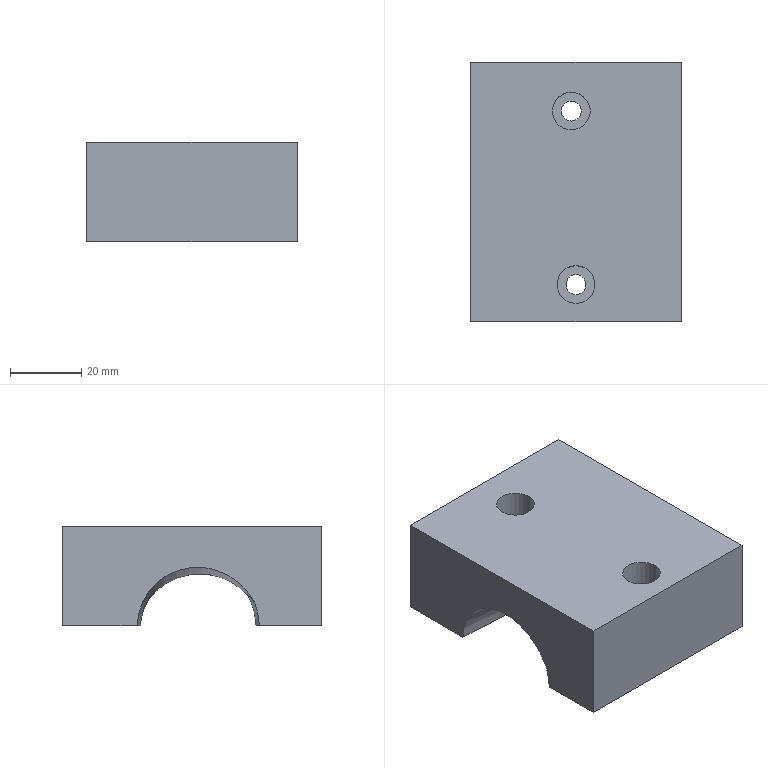NC program | NX | posted with a generic post | part box 59.014 x 72.744 x 27.972 mm
Whole program:
N10 G17 G21 G94 G90
(FLOOR_WALL , TOOL : D63)
N12 T03 M6
N14 G54
N16 G17 G0 G90 X73.872 Y0. S6500 M3
N18 G43 Z30. H3
N20 Z3.
N22 G94 G1 Z0. F1500.
N24 X70.872
N26 X-70.872
N28 X-73.872
N30 Z3.
N32 G0 Z30.
N34 M5
(DRILLING , TOOL : D6A45)
N36 T01 M6
N38 G54
N40 G17 G0 G90 X25.98 Y0. S5000 M3
N42 G43 Z30. H1
N44 G94 G81 G98 Z-1. F250. R3.
N46 X-22.701 Y-1.319
N48 G80
N50 G0 X-22.701 Y-1.319 Z30.
N52 M5
(DRILLING_COPY_COPY , TOOL : 5.6ZT)
N54 T20 M6
N56 G54
N58 G17 G0 G90 X-22.701 Y-1.319 S2000 M3
N60 G43 Z30. H20
N62 G94 G83 G98 Z-31.154 F150. Q3. R3.
N64 X25.98 Y0.
N66 G80
N68 G0 X25.98 Y0. Z30.
N70 M5
(HOLE_MILLING , TOOL : D6)
N72 T16 M6
N74 G54
N76 G17 G0 G90 X-22.701 Y-1.319 S9500 M3
N78 G43 Z30. H16
N80 Z0.5
N82 G94 G3 X-21.551 Y-0.169 R1.15 F1450.
N84 X-22.701 Y0.981 R1.15
N86 X-22.701 Y0.981 Z0. I0. J-2.3
N88 X-22.701 Y0.981 Z-0.5 I0. J-2.3
N90 X-22.701 Y0.981 Z-1. I0. J-2.3
N92 X-22.701 Y0.981 Z-1.5 I0. J-2.3
N94 X-22.701 Y0.981 Z-2. I0. J-2.3
N96 X-22.701 Y0.981 Z-2.5 I0. J-2.3
N98 X-22.701 Y0.981 Z-3. I0. J-2.3
N100 X-22.701 Y0.981 Z-3.5 I0. J-2.3
N102 X-22.701 Y0.981 Z-4. I0. J-2.3
N104 X-22.701 Y0.981 Z-4.5 I0. J-2.3
N106 X-22.701 Y0.981 Z-5. I0. J-2.3
N108 X-22.701 Y0.981 Z-5.5 I0. J-2.3
N110 X-22.701 Y0.981 Z-6. I0. J-2.3
N112 X-22.701 Y0.981 Z-6.5 I0. J-2.3
N114 X-22.701 Y0.981 Z-7. I0. J-2.3
N116 X-22.701 Y0.981 Z-7.5 I0. J-2.3
N118 X-22.701 Y0.981 Z-8. I0. J-2.3
N120 X-22.701 Y0.981 Z-8.5 I0. J-2.3
N122 X-22.701 Y0.981 Z-9. I0. J-2.3
N124 X-22.701 Y0.981 Z-9.5 I0. J-2.3
N126 X-22.701 Y0.981 Z-10. I0. J-2.3
N128 X-22.701 Y0.981 Z-10.5 I0. J-2.3
N130 X-22.701 Y0.981 Z-11. I0. J-2.3
N132 X-22.701 Y0.981 Z-11.5 I0. J-2.3
N134 X-22.701 Y0.981 Z-12. I0. J-2.3
N136 X-22.701 Y0.981 Z-12.5 I0. J-2.3
N138 X-22.701 Y0.981 Z-13. I0. J-2.3
N140 X-22.701 Y0.981 Z-13.5 I0. J-2.3
N142 X-22.701 Y0.981 Z-14. I0. J-2.3
N144 X-22.701 Y0.981 Z-14.5 I0. J-2.3
N146 X-22.701 Y0.981 Z-15. I0. J-2.3
N148 X-22.701 Y0.981 Z-15.5 I0. J-2.3
N150 X-22.701 Y0.981 Z-16. I0. J-2.3
N152 X-22.701 Y0.981 Z-16.5 I0. J-2.3
N154 X-22.701 Y0.981 Z-17. I0. J-2.3
N156 X-22.701 Y0.981 Z-17.5 I0. J-2.3
N158 X-22.701 Y0.981 Z-18. I0. J-2.3
N160 X-22.701 Y0.981 Z-18.5 I0. J-2.3
N162 X-22.701 Y0.981 Z-19. I0. J-2.3
N164 X-22.701 Y0.981 Z-19.5 I0. J-2.3
N166 X-22.701 Y0.981 Z-20. I0. J-2.3
N168 X-25.001 Y-1.319 R2.3
N170 X-22.701 Y0.981 R-2.3
N172 X-23.851 Y-0.169 R1.15
N174 X-22.701 Y-1.319 R1.15
N176 G0 Z30.
N178 X25.98 Y0.
N180 Z0.5
N182 G3 X27.13 Y1.15 R1.15
N184 X25.98 Y2.3 R1.15
N186 X25.98 Y2.3 Z0. I0. J-2.3
N188 X25.98 Y2.3 Z-0.5 I0. J-2.3
N190 X25.98 Y2.3 Z-1. I0. J-2.3
N192 X25.98 Y2.3 Z-1.5 I0. J-2.3
N194 X25.98 Y2.3 Z-2. I0. J-2.3
N196 X25.98 Y2.3 Z-2.5 I0. J-2.3
N198 X25.98 Y2.3 Z-3. I0. J-2.3
N200 X25.98 Y2.3 Z-3.5 I0. J-2.3
N202 X25.98 Y2.3 Z-4. I0. J-2.3
N204 X25.98 Y2.3 Z-4.5 I0. J-2.3
N206 X25.98 Y2.3 Z-5. I0. J-2.3
N208 X25.98 Y2.3 Z-5.5 I0. J-2.3
N210 X25.98 Y2.3 Z-6. I0. J-2.3
N212 X25.98 Y2.3 Z-6.5 I0. J-2.3
N214 X25.98 Y2.3 Z-7. I0. J-2.3
N216 X25.98 Y2.3 Z-7.5 I0. J-2.3
N218 X25.98 Y2.3 Z-8. I0. J-2.3
N220 X25.98 Y2.3 Z-8.5 I0. J-2.3
N222 X25.98 Y2.3 Z-9. I0. J-2.3
N224 X25.98 Y2.3 Z-9.5 I0. J-2.3
N226 X25.98 Y2.3 Z-10. I0. J-2.3
N228 X25.98 Y2.3 Z-10.5 I0. J-2.3
N230 X25.98 Y2.3 Z-11. I0. J-2.3
N232 X25.98 Y2.3 Z-11.5 I0. J-2.3
N234 X25.98 Y2.3 Z-12. I0. J-2.3
N236 X25.98 Y2.3 Z-12.5 I0. J-2.3
N238 X25.98 Y2.3 Z-13. I0. J-2.3
N240 X25.98 Y2.3 Z-13.5 I0. J-2.3
N242 X25.98 Y2.3 Z-14. I0. J-2.3
N244 X25.98 Y2.3 Z-14.5 I0. J-2.3
N246 X25.98 Y2.3 Z-15. I0. J-2.3
N248 X25.98 Y2.3 Z-15.5 I0. J-2.3
N250 X25.98 Y2.3 Z-16. I0. J-2.3
N252 X25.98 Y2.3 Z-16.5 I0. J-2.3
N254 X25.98 Y2.3 Z-17. I0. J-2.3
N256 X25.98 Y2.3 Z-17.5 I0. J-2.3
N258 X25.98 Y2.3 Z-18. I0. J-2.3
N260 X25.98 Y2.3 Z-18.5 I0. J-2.3
N262 X25.98 Y2.3 Z-19. I0. J-2.3
N264 X25.98 Y2.3 Z-19.5 I0. J-2.3
N266 X25.98 Y2.3 Z-20. I0. J-2.3
N268 X23.68 Y0. R2.3
N270 X25.98 Y2.3 R-2.3
N272 X24.83 Y1.15 R1.15
N274 X25.98 Y0. R1.15
N276 G0 Z30.
N278 M5
(ADAPTIVE_MILLING , TOOL : D10)
N280 T04 M6
N282 G54
N284 G17 G0 G90 X0.007 Y-40.226 S9500 M3
N286 G43 Z30. H4
N288 Z-10.986
N290 G94 G1 Z-13.986 F1000.
N292 X0.246 Y-39.385 F3000.
N294 X0.461 Y-38.539
N296 G3 X0.007 Y-37.579 R1.021
N298 X-2.381 Y-36.886 R6.067
N300 X-10.019 Y-36.54 R67.293
N302 G1 X-11.294 Y-36.532
N304 X-12.944 Y-36.525
N306 X-15.269 Y-36.52
N308 X-19.169 Y-36.517
N310 X-32.519 Y-36.515
N312 X-36.344
N314 G2 X-40.675 Y-34.169 R5.616
N316 X-42.848 Y-28.566 R12.027
N318 X-43.324 Y-20.262 R61.031
N320 G1 X-43.334 Y-19.137
N322 X-43.343 Y-17.862
N324 X-43.349 Y-16.137
N326 X-43.354 Y-13.662
N328 X-43.357 Y-9.312
N330 X-43.358 Y13.263
N332 Y29.463
N334 X-43.355 Y29.613
N336 X-43.349 Y29.763
N338 X-43.343 Y29.838
N340 X-43.336 Y29.913
N342 G2 X-40.511 Y34.141 R6.031
N344 X-35.025 Y36.027 R13.154
N346 X-25.892 Y36.469 R72.867
N348 G1 X-24.542 Y36.478
N350 X-22.817 Y36.484
N352 X-20.342 Y36.489
N354 X-16.067 Y36.492
N356 X5.833
N358 X36.358
N360 G2 X40.719 Y34.052 R5.68
N362 X42.838 Y28.504 R12.228
N364 X43.327 Y19.825 R62.853
N366 G1 X43.337 Y18.7
N368 X43.344 Y17.35
N370 X43.351 Y15.475
N372 X43.355 Y12.7
N374 X43.357 Y7.375
N376 X43.358 Y-29.525
N378 G2 X40.951 Y-33.827 R5.679
N380 X35.486 Y-35.956 R12.084
N382 X26.658 Y-36.462 R62.364
N384 G1 X25.459 Y-36.472
N386 X23.959 Y-36.48
N388 X21.934 Y-36.486
N390 X19.009 Y-36.49
N392 X12.934 Y-36.492
N394 X3.784 Y-36.493
N396 G2 X-1.664 Y-35.972 R64.763
N398 G3 X-13.577 Y-35.545 R131.32
N400 G1 X-15.377 Y-35.538
N402 X-17.777 Y-35.532
N404 X-21.527 Y-35.529
N406 X-30.527 Y-35.527
N408 X-33.302
N410 X-33.452 Y-35.525
N412 X-33.527 Y-35.523
N414 X-33.677 Y-35.517
N416 X-33.833 Y-35.507
N418 X-36.342
N420 X-36.401 Y-35.504
N422 G2 X-41.095 Y-33.197 R6.23
N424 X-42.372 Y-29.477 R6.482
N426 G1 Y29.477
N428 X-42.368 Y29.537
N430 G2 X-40.062 Y34.23 R6.23
N432 X-36.342 Y35.507 R6.482
N434 G1 X36.342
N436 X36.401 Y35.504
N438 G2 X41.095 Y33.197 R6.23
N440 X42.372 Y29.477 R6.482
N442 G1 Y-29.477
N444 X42.368 Y-29.537
N446 G2 X40.062 Y-34.23 R6.23
N448 X36.342 Y-35.507 R6.482
N450 G1 X-33.858
N452 G3 X-34.648 Y-35.888 R1.026
N454 G1 X-36.336 Y-38.007
N456 Z-10.986
N458 G0 Z30.
N460 X0.009 Y-40.228
N462 Z-24.972
N464 G1 Z-27.972 F1000.
N466 X0.248 Y-39.387 F3000.
N468 X0.463 Y-38.541
N470 G3 X0.009 Y-37.581 R1.021
N472 X-2.38 Y-36.887 R6.067
N474 X-10.017 Y-36.542 R67.293
N476 G1 X-11.292 Y-36.533
N478 X-12.942 Y-36.526
N480 X-15.267 Y-36.521
N482 X-19.167 Y-36.518
N484 X-32.517 Y-36.517
N486 X-36.342
N488 G2 X-40.674 Y-34.174 R5.603
N490 X-42.821 Y-28.718 R11.888
N492 X-43.329 Y-19.966 R61.091
N494 G1 X-43.339 Y-18.766
N496 X-43.347 Y-17.341
N498 X-43.353 Y-15.466
N500 X-43.357 Y-12.616
N502 X-43.359 Y-6.991
N504 Y29.534
N506 G2 X-40.944 Y33.832 R5.701
N508 X-35.477 Y35.958 R12.124
N510 X-27.25 Y36.458 R58.169
N512 G1 X-26.2 Y36.469
N514 X-25. Y36.477
N516 X-23.35 Y36.484
N518 X-21.175 Y36.49
N520 X-17.65 Y36.493
N522 X-7.975 Y36.494
N524 X36.35
N526 X36.5 Y36.492
N528 X36.575 Y36.488
N530 X36.725 Y36.478
N532 X36.799 Y36.471
N534 G2 X40.978 Y33.695 R6.032
N536 X42.918 Y27.995 R13.288
N538 X43.337 Y19.01 R75.636
N540 G1 X43.345 Y17.66
N542 X43.351 Y15.86
N544 X43.356 Y13.31
N546 X43.359 Y8.735
N548 Y-22.465
N550 Y-29.515
N552 G2 X40.961 Y-33.821 R5.68
N554 X35.498 Y-35.956 R12.099
N556 X27.57 Y-36.454 R56.423
N558 G1 X26.595 Y-36.465
N560 X25.471 Y-36.474
N562 X23.971 Y-36.482
N564 X22.021 Y-36.488
N566 X19.096 Y-36.492
N568 X13.021 Y-36.494
N570 G2 X2.672 Y-36.449 R304.437
N572 G3 X-5.017 Y-35.722 R165.027
N574 X-19.34 Y-35.532 R354.213
N576 G1 X-24.44 Y-35.529
N578 X-33.29
N580 X-33.44 Y-35.527
N582 X-33.59 Y-35.522
N584 X-33.74 Y-35.515
N586 X-33.854 Y-35.507
N588 X-36.342
N590 X-36.401 Y-35.504
N592 G2 X-41.095 Y-33.197 R6.23
N594 X-42.372 Y-29.477 R6.482
N596 G1 Y29.477
N598 X-42.368 Y29.537
N600 G2 X-40.062 Y34.23 R6.23
N602 X-36.342 Y35.507 R6.482
N604 G1 X36.342
N606 X36.401 Y35.504
N608 G2 X41.095 Y33.197 R6.23
N610 X42.372 Y29.477 R6.482
N612 G1 Y-29.477
N614 X42.368 Y-29.537
N616 G2 X40.062 Y-34.23 R6.23
N618 X36.342 Y-35.507 R6.482
N620 G1 X-33.858
N622 G3 X-34.648 Y-35.888 R1.026
N624 G1 X-36.336 Y-38.007
N626 Z-24.972
N628 G0 Z30.
N630 M5
(ZLEVEL_PROFILE_COPY_COPY , TOOL : D10JING)
N632 T14 M6
N634 G54
N636 G17 G0 G90 X37.468 Y-35.406 S9500 M3
N638 G43 Z30. H14
N640 Z-13.986
N642 G94 G1 X37.238 Y-35.007 F1000.
N644 G3 X36.372 Y-34.507 R1.
N646 G1 X-36.372 F1200.
N648 G2 X-41.372 Y-29.507 R5.
N650 G1 Y29.507
N652 G2 X-36.372 Y34.507 R5.
N654 G1 X36.372
N656 G2 X41.372 Y29.507 R5.
N658 G1 Y-29.507
N660 G2 X36.372 Y-34.507 R5.
N662 G3 X35.506 Y-35.007 R1.
N664 G1 X35.217 Y-35.507
N666 G0 X37.468 Y-35.406 Z-27.972
N668 G1 X37.238 Y-35.007 F1000.
N670 G3 X36.372 Y-34.507 R1.
N672 G1 X-36.372 F1200.
N674 G2 X-41.372 Y-29.507 R5.
N676 G1 Y29.507
N678 G2 X-36.372 Y34.507 R5.
N680 G1 X36.372
N682 G2 X41.372 Y29.507 R5.
N684 G1 Y-29.507
N686 G2 X36.372 Y-34.507 R5.
N688 G3 X35.506 Y-35.007 R1.
N690 G1 X35.217 Y-35.507
N692 G0 Z30.
N694 M5
(ZLEVEL_PROFILE_1 , TOOL : D6A45)
N696 T01 M6
N698 G54
N700 G17 G0 G90 X28.896 Y-1.17 S9500 M3
N702 G43 Z30. H1
N704 Z0.5
N706 G94 G1 Z-1. F1250.
N708 X30.022 Y-0.52
N710 G3 X30.322 Y0. R0.6
N712 X25.98 Y4.341 R4.341
N714 X30.322 Y0. R-4.341
N716 X30.022 Y0.52 R0.6
N718 G1 X28.896 Y1.17
N720 Z0.5
N722 G0 Z30.
N724 X-25.616 Y-0.15
N726 Z0.5
N728 G1 Z-1.
N730 X-26.742 Y-0.8
N732 G3 X-27.042 Y-1.319 R0.6
N734 X-22.701 Y-5.661 R4.341
N736 X-27.042 Y-1.319 R-4.341
N738 X-26.742 Y-1.839 R0.6
N740 G1 X-25.616 Y-2.489
N742 Z0.5
N744 G0 Z30.
N746 X-1.039 Y31.666
N748 Z0.5
N750 G1 Z-1.
N752 X-0.52 Y30.766
N754 G3 X0. Y30.466 R0.6
N756 G1 X36.374
N758 G2 X37.33 Y29.518 R0.952
N760 G1 Y-29.51
N762 G2 X36.374 Y-30.466 R0.979
N764 G1 X-36.374
N766 G2 X-37.33 Y-29.51 R0.979
N768 G1 Y29.518
N770 G2 X-36.374 Y30.466 R0.952
N772 G1 X0.
N774 G3 X0.52 Y30.766 R0.6
N776 G1 X1.039 Y31.666
N778 Z0.5
N780 G0 Z30.
N782 M5
N784 M2